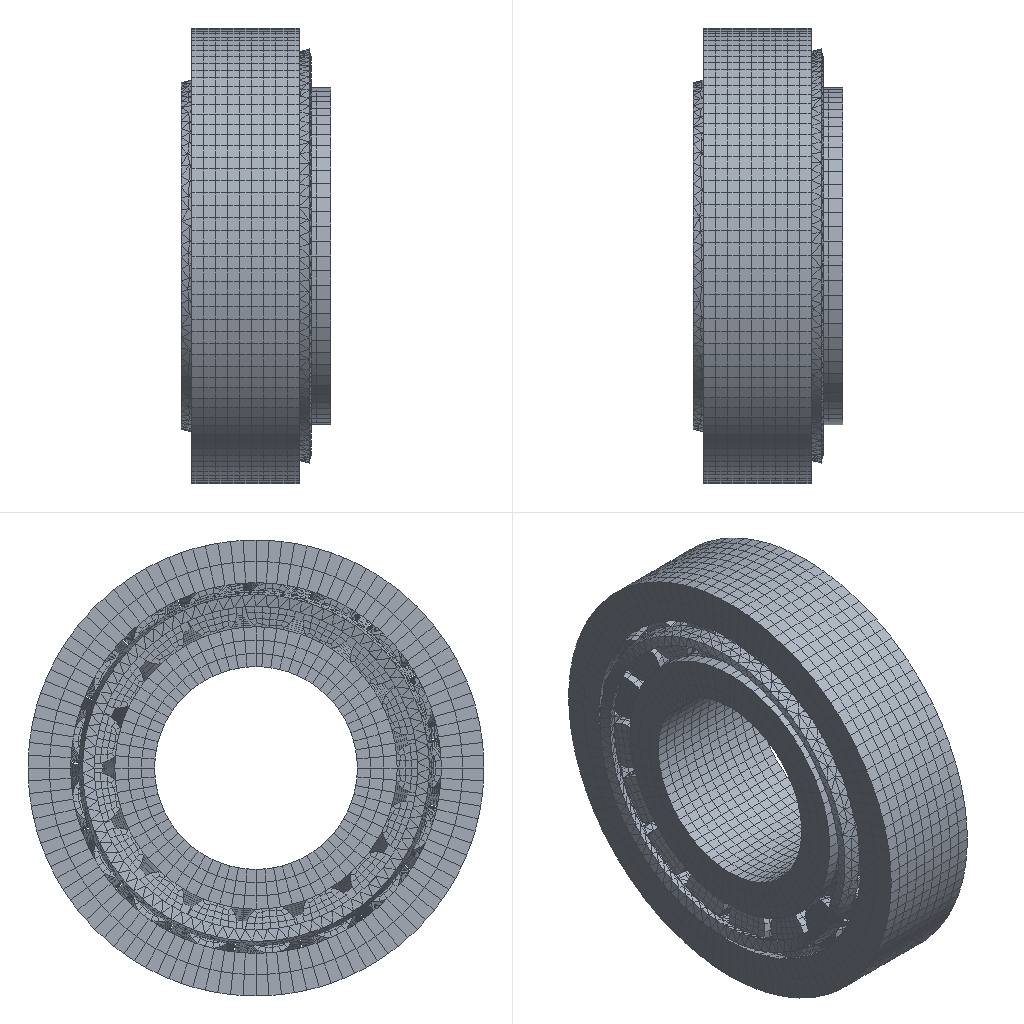Simulation study | abaqus
Set-up summary:
category,name,step,type,value,unit,region
solver,abaqus
solver,version,,,Abaqus/Explicit 2020
units,not stated in the deck,,not stated
analysis,deck,,transient,transient
load_step,Step-1,Step-1,transient
load_step,Step-2,Step-2,transient
load_step,Step-3,Step-3,transient
load_step,requested,,,3
mesh,nodes,,,23189
mesh,elements,,,18827
element_type,C3D4,,solid,3343
element_type,C3D8R,,solid,15484
load,load commands in deck,,count,4
bc,support commands in deck,,count,27
material,CAILIAO1,,in results
check,setup vs results,,match,"per instance, exact: element labels, types and connectivity; labels of the nodes the elements use; coordinates not compared"
Abaqus input file, long lists of numbers shortened:
*Heading
** Job name: Job-2 Model name: Model-1
** Generated by: Abaqus/CAE 2020
*Preprint, echo=NO, model=NO, history=NO, contact=NO
**
** PARTS
**
*Part, name=SKF_15578_15520_3
*Node
      1,   13.495,  -26.339,           0.
      2,   13.495,  -28.575,           0.
** (3358 more lines like these left out)
*Element, type=C3D8R
  1,  147, 1007, 2497,  575,    1,   20,  521,   75
  2, 1007,  156,  791, 2497,   20,    2,   21,  521
** (2014 more lines like these left out)
*Nset, nset=_PickedSet8, internal, generate
    1,  3360,     1
*Elset, elset=_PickedSet8, internal, generate
    1,  2016,     1
** Section: waiquan
*Solid Section, elset=_PickedSet8, material=cailiao1
,
*End Part
**
*Part, name=SKF_15578_15520_5
*Node
      1,   1.787,   17.127,           0.
      2,   1.169,   20.239,           0.
** (768 more lines like these left out)
*Element, type=C3D8R
  1, 165, 166, 498, 489,  13,  14, 124, 123
  2, 166,  18, 129, 498,  14,   1,  15, 124
** (570 more lines like these left out)
*Nset, nset=_PickedSet6, internal, generate
   1,  770,    1
*Elset, elset=_PickedSet6, internal, generate
   1,  572,    1
** Section: gongdongti
*Solid Section, elset=_PickedSet6, material=cailiao1
,
*End Part
**
*Part, name=SKF_15578_15520_23
*Node
      1,  0.7326,  -1.611,  -21.171
      2,  0.6985,           0.,  -21.223
** (1697 more lines like these left out)
*Element, type=C3D4
   1, 1652, 1601, 1637,  503
   2, 1652, 1404, 1405, 1601
** (3341 more lines like these left out)
*Nset, nset=_PickedSet6, internal, generate
    1,  1699,     1
*Elset, elset=_PickedSet6, internal, generate
    1,  3343,     1
** Section: baochijia
*Solid Section, elset=_PickedSet6, material=cailiao1
,
*End Part
**
*Part, name=SKF_15578_15520_25
*Node
      1,   13.796,   21.15,           0.
      2,   14.245,   19.205,           0.
** (5038 more lines like these left out)
*Element, type=C3D8R
  1,    2,  683,   62,    1,  163, 2595,  753,   63
  2,   57,   58,  702,  715,  770,  771, 2614, 2627
** (3742 more lines like these left out)
*Nset, nset=_PickedSet9, internal, generate
    1,  5040,     1
*Elset, elset=_PickedSet9, internal, generate
    1,  3744,     1
** Section: niequan
*Solid Section, elset=_PickedSet9, material=cailiao1
,
*End Part
**
**
** ASSEMBLY
**
*Assembly, name=Assembly
**
*Instance, name=SKF_15578_15520_25, part=SKF_15578_15520_25
          0.,           0.,           0.
          0.,           0.,           0.,           1.,           0.,           0.,         180.
*End Instance
**
*Instance, name=SKF_15578_15520_23, part=SKF_15578_15520_23
          0.,           0.,           0.
          0.,           0.,           0.,           1.,           0.,           0.,         180.
*End Instance
**
*Instance, name=SKF_15578_15520_5, part=SKF_15578_15520_5
          0.,           0.,           0.
          0.,           0.,           0.,           1.,           0.,           0.,         180.
*End Instance
**
*Instance, name=SKF_15578_15520_5_1, part=SKF_15578_15520_5
          0.,           0.,           0.
          0.,           0.,           0., 1.,           0.,           0., 201.176
*End Instance
**
*Instance, name=SKF_15578_15520_5_2, part=SKF_15578_15520_5
          0.,           0.,           0.
          0.,           0.,           0., 1.,           0.,           0., 222.353
*End Instance
**
*Instance, name=SKF_15578_15520_5_3, part=SKF_15578_15520_5
          0.,           0.,           0.
          0.,           0.,           0., -1.,           0.,           0., 116.471
*End Instance
**
*Instance, name=SKF_15578_15520_5_4, part=SKF_15578_15520_5
          0.,           0.,           0.
          0.,           0.,           0., -1.,           0.,           0., 95.294
*End Instance
**
*Instance, name=SKF_15578_15520_5_5, part=SKF_15578_15520_5
          0.,           0.,           0.
          0.,           0.,           0., -1.,           0.,           0., 74.118
*End Instance
**
*Instance, name=SKF_15578_15520_5_6, part=SKF_15578_15520_5
          0.,           0.,           0.
          0.,           0.,           0., -1.,           0.,           0., 52.941
*End Instance
**
*Instance, name=SKF_15578_15520_5_7, part=SKF_15578_15520_5
          0.,           0.,           0.
          0.,           0.,           0., -1.,           0.,           0., 31.765
*End Instance
**
*Instance, name=SKF_15578_15520_5_8, part=SKF_15578_15520_5
          0.,           0.,           0.
          0.,           0.,           0., -1.,           0.,           0., 10.588
*End Instance
**
*Instance, name=SKF_15578_15520_5_9, part=SKF_15578_15520_5
          0.,           0.,           0.
          0.,           0.,           0., 1.,           0.,           0., 10.588
*End Instance
**
*Instance, name=SKF_15578_15520_5_10, part=SKF_15578_15520_5
          0.,           0.,           0.
          0.,           0.,           0., 1.,           0.,           0., 31.765
*End Instance
**
*Instance, name=SKF_15578_15520_5_11, part=SKF_15578_15520_5
          0.,           0.,           0.
          0.,           0.,           0., 1.,           0.,           0., 52.941
*End Instance
**
*Instance, name=SKF_15578_15520_5_12, part=SKF_15578_15520_5
          0.,           0.,           0.
          0.,           0.,           0., 1.,           0.,           0., 74.118
*End Instance
**
*Instance, name=SKF_15578_15520_5_13, part=SKF_15578_15520_5
          0.,           0.,           0.
          0.,           0.,           0., 1.,           0.,           0., 95.294
*End Instance
**
*Instance, name=SKF_15578_15520_5_14, part=SKF_15578_15520_5
          0.,           0.,           0.
          0.,           0.,           0., 1.,           0.,           0., 116.471
*End Instance
**
*Instance, name=SKF_15578_15520_5_15, part=SKF_15578_15520_5
          0.,           0.,           0.
          0.,           0.,           0., 1.,           0.,           0., 137.647
*End Instance
**
*Instance, name=SKF_15578_15520_5_16, part=SKF_15578_15520_5
          0.,           0.,           0.
          0.,           0.,           0., 1.,           0.,           0., 158.824
*End Instance
**
*Instance, name=SKF_15578_15520_3, part=SKF_15578_15520_3
          0.,           0.,           0.
          0.,           0.,           0.,           1.,           0.,           0.,         180.
*End Instance
**
*Node
      1,   17.462, -4.4408921e-15,           0.
*Node
      2,   14.245, 2.9840975e-15,           0.
*Node
      3,           0.,           0.,          40.
*Node
      4,           0.,           0.,           0.
*Node
      5,   7.122, 1.49204875e-15,           0.
*Nset, nset=Set-7, instance=SKF_15578_15520_23
    6,    7,  110,  111,  152,  153,  154,  169,  170,  171,  172,  173,  174,  175,  176,  177
  178,  179,  180,  181,  182,  183,  184,  185,  186,  187,  188,  189,  190,  191,  192,  193
** (23 more lines like these left out)
*Elset, elset=Set-7, instance=SKF_15578_15520_23
    3,   46,   72,   81,   99,  106,  125,  222,  230,  238,  253,  273,  282,  289,  291,  293
  296,  297,  298,  301,  302,  304,  308,  319,  320,  325,  328,  329,  339,  341,  342,  348
** (23 more lines like these left out)
*Nset, nset=Set-8
 4,
*Nset, nset=Set-9
 2,
*Nset, nset=Set-10
 5,
*Nset, nset=m_Set-1
 1,
*Nset, nset=m_Set-8
 4,
*Nset, nset=m_Set-9
 2,
*Nset, nset=m_Set-10
 5,
*Nset, nset=ouhe-holder, instance=SKF_15578_15520_23, generate
    1,  1699,     1
*Elset, elset=ouhe-holder, instance=SKF_15578_15520_23, generate
    1,  3343,     1
*Nset, nset=_PickedSet53, internal
 2,
*Elset, elset=_Surf-1_S4, internal, instance=SKF_15578_15520_5_5
  49,  50,  51,  52,  53,  54,  55,  56,  57,  58,  59,  60,  61,  62,  63,  64
  65,  66,  73,  80, 192, 193, 194, 195, 196, 197, 198, 199, 200, 201, 202, 203
** (7 more lines like these left out)
*Elset, elset=_Surf-1_S3, internal, instance=SKF_15578_15520_5_5
   1,   2,   3,   4,   5,   6,   7,   8,   9,  10,  11,  12,  67,  68,  69,  70
  71,  72,  73,  74,  75,  76,  77,  78,  79,  80,  81,  82,  83, 102, 103, 104
** (9 more lines like these left out)
*Elset, elset=_Surf-1_S2, internal, instance=SKF_15578_15520_5_5
   1,   2,  13,  14,  15,  16,  17,  18,  49,  50,  51, 123, 124, 125, 144, 145
 156, 157, 158, 159, 160, 161, 192, 193, 194, 287, 288, 299, 300, 301, 302, 303
** (1 more lines like these left out)
*Surface, type=ELEMENT, name=Surf-1
_Surf-1_S4, S4
_Surf-1_S3, S3
_Surf-1_S2, S2
*Elset, elset=_Surf-2_S4, internal, instance=SKF_15578_15520_5_6
  49,  50,  51,  52,  53,  54,  55,  56,  57,  58,  59,  60,  61,  62,  63,  64
  65,  66,  73,  80, 192, 193, 194, 195, 196, 197, 198, 199, 200, 201, 202, 203
** (7 more lines like these left out)
*Elset, elset=_Surf-2_S3, internal, instance=SKF_15578_15520_5_6
   1,   2,   3,   4,   5,   6,   7,   8,   9,  10,  11,  12,  67,  68,  69,  70
  71,  72,  73,  74,  75,  76,  77,  78,  79,  80,  81,  82,  83, 102, 103, 104
** (9 more lines like these left out)
*Elset, elset=_Surf-2_S2, internal, instance=SKF_15578_15520_5_6
   1,   2,  13,  14,  15,  16,  17,  18,  49,  50,  51, 123, 124, 125, 144, 145
 156, 157, 158, 159, 160, 161, 192, 193, 194, 287, 288, 299, 300, 301, 302, 303
** (1 more lines like these left out)
*Surface, type=ELEMENT, name=Surf-2
_Surf-2_S4, S4
_Surf-2_S3, S3
_Surf-2_S2, S2
*Elset, elset=_Surf-3_S4, internal, instance=SKF_15578_15520_5_7
  49,  50,  51,  52,  53,  54,  55,  56,  57,  58,  59,  60,  61,  62,  63,  64
  65,  66,  73,  80, 192, 193, 194, 195, 196, 197, 198, 199, 200, 201, 202, 203
** (7 more lines like these left out)
*Elset, elset=_Surf-3_S3, internal, instance=SKF_15578_15520_5_7
   1,   2,   3,   4,   5,   6,   7,   8,   9,  10,  11,  12,  67,  68,  69,  70
  71,  72,  73,  74,  75,  76,  77,  78,  79,  80,  81,  82,  83, 102, 103, 104
** (9 more lines like these left out)
*Elset, elset=_Surf-3_S2, internal, instance=SKF_15578_15520_5_7
   1,   2,  13,  14,  15,  16,  17,  18,  49,  50,  51, 123, 124, 125, 144, 145
 156, 157, 158, 159, 160, 161, 192, 193, 194, 287, 288, 299, 300, 301, 302, 303
** (1 more lines like these left out)
*Surface, type=ELEMENT, name=Surf-3
_Surf-3_S4, S4
_Surf-3_S3, S3
_Surf-3_S2, S2
*Elset, elset=_Surf-4_S4, internal, instance=SKF_15578_15520_5_8
  49,  50,  51,  52,  53,  54,  55,  56,  57,  58,  59,  60,  61,  62,  63,  64
  65,  66,  73,  80, 192, 193, 194, 195, 196, 197, 198, 199, 200, 201, 202, 203
** (7 more lines like these left out)
*Elset, elset=_Surf-4_S3, internal, instance=SKF_15578_15520_5_8
   1,   2,   3,   4,   5,   6,   7,   8,   9,  10,  11,  12,  67,  68,  69,  70
  71,  72,  73,  74,  75,  76,  77,  78,  79,  80,  81,  82,  83, 102, 103, 104
** (9 more lines like these left out)
*Elset, elset=_Surf-4_S2, internal, instance=SKF_15578_15520_5_8
   1,   2,  13,  14,  15,  16,  17,  18,  49,  50,  51, 123, 124, 125, 144, 145
 156, 157, 158, 159, 160, 161, 192, 193, 194, 287, 288, 299, 300, 301, 302, 303
** (1 more lines like these left out)
*Surface, type=ELEMENT, name=Surf-4
_Surf-4_S4, S4
_Surf-4_S3, S3
_Surf-4_S2, S2
*Elset, elset=_Surf-5_S4, internal, instance=SKF_15578_15520_5_9
  49,  50,  51,  52,  53,  54,  55,  56,  57,  58,  59,  60,  61,  62,  63,  64
  65,  66,  73,  80, 192, 193, 194, 195, 196, 197, 198, 199, 200, 201, 202, 203
** (7 more lines like these left out)
*Elset, elset=_Surf-5_S3, internal, instance=SKF_15578_15520_5_9
   1,   2,   3,   4,   5,   6,   7,   8,   9,  10,  11,  12,  67,  68,  69,  70
  71,  72,  73,  74,  75,  76,  77,  78,  79,  80,  81,  82,  83, 102, 103, 104
** (9 more lines like these left out)
*Elset, elset=_Surf-5_S2, internal, instance=SKF_15578_15520_5_9
   1,   2,  13,  14,  15,  16,  17,  18,  49,  50,  51, 123, 124, 125, 144, 145
 156, 157, 158, 159, 160, 161, 192, 193, 194, 287, 288, 299, 300, 301, 302, 303
** (1 more lines like these left out)
*Surface, type=ELEMENT, name=Surf-5
_Surf-5_S4, S4
_Surf-5_S3, S3
_Surf-5_S2, S2
*Elset, elset=_Surf-6_S4, internal, instance=SKF_15578_15520_5_10
  49,  50,  51,  52,  53,  54,  55,  56,  57,  58,  59,  60,  61,  62,  63,  64
  65,  66,  73,  80, 192, 193, 194, 195, 196, 197, 198, 199, 200, 201, 202, 203
** (7 more lines like these left out)
*Elset, elset=_Surf-6_S3, internal, instance=SKF_15578_15520_5_10
   1,   2,   3,   4,   5,   6,   7,   8,   9,  10,  11,  12,  67,  68,  69,  70
  71,  72,  73,  74,  75,  76,  77,  78,  79,  80,  81,  82,  83, 102, 103, 104
** (9 more lines like these left out)
*Elset, elset=_Surf-6_S2, internal, instance=SKF_15578_15520_5_10
   1,   2,  13,  14,  15,  16,  17,  18,  49,  50,  51, 123, 124, 125, 144, 145
 156, 157, 158, 159, 160, 161, 192, 193, 194, 287, 288, 299, 300, 301, 302, 303
** (1 more lines like these left out)
*Surface, type=ELEMENT, name=Surf-6
_Surf-6_S4, S4
_Surf-6_S3, S3
_Surf-6_S2, S2
*Elset, elset=_Surf-7_S4, internal, instance=SKF_15578_15520_5_11
  49,  50,  51,  52,  53,  54,  55,  56,  57,  58,  59,  60,  61,  62,  63,  64
  65,  66,  73,  80, 192, 193, 194, 195, 196, 197, 198, 199, 200, 201, 202, 203
** (7 more lines like these left out)
*Elset, elset=_Surf-7_S3, internal, instance=SKF_15578_15520_5_11
   1,   2,   3,   4,   5,   6,   7,   8,   9,  10,  11,  12,  67,  68,  69,  70
  71,  72,  73,  74,  75,  76,  77,  78,  79,  80,  81,  82,  83, 102, 103, 104
** (9 more lines like these left out)
*Elset, elset=_Surf-7_S2, internal, instance=SKF_15578_15520_5_11
   1,   2,  13,  14,  15,  16,  17,  18,  49,  50,  51, 123, 124, 125, 144, 145
 156, 157, 158, 159, 160, 161, 192, 193, 194, 287, 288, 299, 300, 301, 302, 303
** (1 more lines like these left out)
*Surface, type=ELEMENT, name=Surf-7
_Surf-7_S4, S4
_Surf-7_S3, S3
_Surf-7_S2, S2
*Elset, elset=_Surf-8_S4, internal, instance=SKF_15578_15520_5_12
  49,  50,  51,  52,  53,  54,  55,  56,  57,  58,  59,  60,  61,  62,  63,  64
  65,  66,  73,  80, 192, 193, 194, 195, 196, 197, 198, 199, 200, 201, 202, 203
** (7 more lines like these left out)
*Elset, elset=_Surf-8_S3, internal, instance=SKF_15578_15520_5_12
   1,   2,   3,   4,   5,   6,   7,   8,   9,  10,  11,  12,  67,  68,  69,  70
  71,  72,  73,  74,  75,  76,  77,  78,  79,  80,  81,  82,  83, 102, 103, 104
** (9 more lines like these left out)
*Elset, elset=_Surf-8_S2, internal, instance=SKF_15578_15520_5_12
   1,   2,  13,  14,  15,  16,  17,  18,  49,  50,  51, 123, 124, 125, 144, 145
 156, 157, 158, 159, 160, 161, 192, 193, 194, 287, 288, 299, 300, 301, 302, 303
** (1 more lines like these left out)
*Surface, type=ELEMENT, name=Surf-8
_Surf-8_S4, S4
_Surf-8_S3, S3
_Surf-8_S2, S2
*Elset, elset=_Surf-9_S4, internal, instance=SKF_15578_15520_5_13
  49,  50,  51,  52,  53,  54,  55,  56,  57,  58,  59,  60,  61,  62,  63,  64
  65,  66,  73,  80, 192, 193, 194, 195, 196, 197, 198, 199, 200, 201, 202, 203
** (7 more lines like these left out)
*Elset, elset=_Surf-9_S3, internal, instance=SKF_15578_15520_5_13
   1,   2,   3,   4,   5,   6,   7,   8,   9,  10,  11,  12,  67,  68,  69,  70
  71,  72,  73,  74,  75,  76,  77,  78,  79,  80,  81,  82,  83, 102, 103, 104
** (9 more lines like these left out)
*Elset, elset=_Surf-9_S2, internal, instance=SKF_15578_15520_5_13
   1,   2,  13,  14,  15,  16,  17,  18,  49,  50,  51, 123, 124, 125, 144, 145
 156, 157, 158, 159, 160, 161, 192, 193, 194, 287, 288, 299, 300, 301, 302, 303
** (1 more lines like these left out)
*Surface, type=ELEMENT, name=Surf-9
_Surf-9_S4, S4
_Surf-9_S3, S3
_Surf-9_S2, S2
*Elset, elset=_Surf-10_S4, internal, instance=SKF_15578_15520_5_14
  49,  50,  51,  52,  53,  54,  55,  56,  57,  58,  59,  60,  61,  62,  63,  64
  65,  66,  73,  80, 192, 193, 194, 195, 196, 197, 198, 199, 200, 201, 202, 203
** (7 more lines like these left out)
*Elset, elset=_Surf-10_S3, internal, instance=SKF_15578_15520_5_14
   1,   2,   3,   4,   5,   6,   7,   8,   9,  10,  11,  12,  67,  68,  69,  70
  71,  72,  73,  74,  75,  76,  77,  78,  79,  80,  81,  82,  83, 102, 103, 104
** (9 more lines like these left out)
*Elset, elset=_Surf-10_S2, internal, instance=SKF_15578_15520_5_14
   1,   2,  13,  14,  15,  16,  17,  18,  49,  50,  51, 123, 124, 125, 144, 145
 156, 157, 158, 159, 160, 161, 192, 193, 194, 287, 288, 299, 300, 301, 302, 303
** (1 more lines like these left out)
*Surface, type=ELEMENT, name=Surf-10
_Surf-10_S4, S4
_Surf-10_S3, S3
_Surf-10_S2, S2
*Elset, elset=_Surf-11_S4, internal, instance=SKF_15578_15520_5_15
  49,  50,  51,  52,  53,  54,  55,  56,  57,  58,  59,  60,  61,  62,  63,  64
  65,  66,  73,  80, 192, 193, 194, 195, 196, 197, 198, 199, 200, 201, 202, 203
** (7 more lines like these left out)
*Elset, elset=_Surf-11_S3, internal, instance=SKF_15578_15520_5_15
   1,   2,   3,   4,   5,   6,   7,   8,   9,  10,  11,  12,  67,  68,  69,  70
  71,  72,  73,  74,  75,  76,  77,  78,  79,  80,  81,  82,  83, 102, 103, 104
** (9 more lines like these left out)
*Elset, elset=_Surf-11_S2, internal, instance=SKF_15578_15520_5_15
   1,   2,  13,  14,  15,  16,  17,  18,  49,  50,  51, 123, 124, 125, 144, 145
 156, 157, 158, 159, 160, 161, 192, 193, 194, 287, 288, 299, 300, 301, 302, 303
** (1 more lines like these left out)
*Surface, type=ELEMENT, name=Surf-11
_Surf-11_S4, S4
_Surf-11_S3, S3
_Surf-11_S2, S2
*Elset, elset=_Surf-12_S4, internal, instance=SKF_15578_15520_5_16
  49,  50,  51,  52,  53,  54,  55,  56,  57,  58,  59,  60,  61,  62,  63,  64
  65,  66,  73,  80, 192, 193, 194, 195, 196, 197, 198, 199, 200, 201, 202, 203
** (7 more lines like these left out)
*Elset, elset=_Surf-12_S3, internal, instance=SKF_15578_15520_5_16
   1,   2,   3,   4,   5,   6,   7,   8,   9,  10,  11,  12,  67,  68,  69,  70
  71,  72,  73,  74,  75,  76,  77,  78,  79,  80,  81,  82,  83, 102, 103, 104
** (9 more lines like these left out)
*Elset, elset=_Surf-12_S2, internal, instance=SKF_15578_15520_5_16
   1,   2,  13,  14,  15,  16,  17,  18,  49,  50,  51, 123, 124, 125, 144, 145
 156, 157, 158, 159, 160, 161, 192, 193, 194, 287, 288, 299, 300, 301, 302, 303
** (1 more lines like these left out)
*Surface, type=ELEMENT, name=Surf-12
_Surf-12_S4, S4
_Surf-12_S3, S3
_Surf-12_S2, S2
*Elset, elset=_Surf-13_S4, internal, instance=SKF_15578_15520_5
  49,  50,  51,  52,  53,  54,  55,  56,  57,  58,  59,  60,  61,  62,  63,  64
  65,  66,  73,  80, 192, 193, 194, 195, 196, 197, 198, 199, 200, 201, 202, 203
** (7 more lines like these left out)
*Elset, elset=_Surf-13_S3, internal, instance=SKF_15578_15520_5
   1,   2,   3,   4,   5,   6,   7,   8,   9,  10,  11,  12,  67,  68,  69,  70
  71,  72,  73,  74,  75,  76,  77,  78,  79,  80,  81,  82,  83, 102, 103, 104
** (9 more lines like these left out)
*Elset, elset=_Surf-13_S2, internal, instance=SKF_15578_15520_5
   1,   2,  13,  14,  15,  16,  17,  18,  49,  50,  51, 123, 124, 125, 144, 145
 156, 157, 158, 159, 160, 161, 192, 193, 194, 287, 288, 299, 300, 301, 302, 303
** (1 more lines like these left out)
*Surface, type=ELEMENT, name=Surf-13
_Surf-13_S4, S4
_Surf-13_S3, S3
_Surf-13_S2, S2
*Elset, elset=_Surf-14_S4, internal, instance=SKF_15578_15520_5_1
  49,  50,  51,  52,  53,  54,  55,  56,  57,  58,  59,  60,  61,  62,  63,  64
  65,  66,  73,  80, 192, 193, 194, 195, 196, 197, 198, 199, 200, 201, 202, 203
** (7 more lines like these left out)
*Elset, elset=_Surf-14_S3, internal, instance=SKF_15578_15520_5_1
   1,   2,   3,   4,   5,   6,   7,   8,   9,  10,  11,  12,  67,  68,  69,  70
  71,  72,  73,  74,  75,  76,  77,  78,  79,  80,  81,  82,  83, 102, 103, 104
** (9 more lines like these left out)
*Elset, elset=_Surf-14_S2, internal, instance=SKF_15578_15520_5_1
   1,   2,  13,  14,  15,  16,  17,  18,  49,  50,  51, 123, 124, 125, 144, 145
 156, 157, 158, 159, 160, 161, 192, 193, 194, 287, 288, 299, 300, 301, 302, 303
** (1 more lines like these left out)
*Surface, type=ELEMENT, name=Surf-14
_Surf-14_S4, S4
_Surf-14_S3, S3
_Surf-14_S2, S2
*Elset, elset=_Surf-15_S4, internal, instance=SKF_15578_15520_5_2
  49,  50,  51,  52,  53,  54,  55,  56,  57,  58,  59,  60,  61,  62,  63,  64
  65,  66,  73,  80, 192, 193, 194, 195, 196, 197, 198, 199, 200, 201, 202, 203
** (7 more lines like these left out)
*Elset, elset=_Surf-15_S3, internal, instance=SKF_15578_15520_5_2
   1,   2,   3,   4,   5,   6,   7,   8,   9,  10,  11,  12,  67,  68,  69,  70
  71,  72,  73,  74,  75,  76,  77,  78,  79,  80,  81,  82,  83, 102, 103, 104
** (9 more lines like these left out)
*Elset, elset=_Surf-15_S2, internal, instance=SKF_15578_15520_5_2
   1,   2,  13,  14,  15,  16,  17,  18,  49,  50,  51, 123, 124, 125, 144, 145
 156, 157, 158, 159, 160, 161, 192, 193, 194, 287, 288, 299, 300, 301, 302, 303
** (1 more lines like these left out)
*Surface, type=ELEMENT, name=Surf-15
_Surf-15_S4, S4
_Surf-15_S3, S3
_Surf-15_S2, S2
*Elset, elset=_Surf-16_S4, internal, instance=SKF_15578_15520_5_3
  49,  50,  51,  52,  53,  54,  55,  56,  57,  58,  59,  60,  61,  62,  63,  64
  65,  66,  73,  80, 192, 193, 194, 195, 196, 197, 198, 199, 200, 201, 202, 203
** (7 more lines like these left out)
*Elset, elset=_Surf-16_S3, internal, instance=SKF_15578_15520_5_3
   1,   2,   3,   4,   5,   6,   7,   8,   9,  10,  11,  12,  67,  68,  69,  70
  71,  72,  73,  74,  75,  76,  77,  78,  79,  80,  81,  82,  83, 102, 103, 104
** (9 more lines like these left out)
*Elset, elset=_Surf-16_S2, internal, instance=SKF_15578_15520_5_3
   1,   2,  13,  14,  15,  16,  17,  18,  49,  50,  51, 123, 124, 125, 144, 145
 156, 157, 158, 159, 160, 161, 192, 193, 194, 287, 288, 299, 300, 301, 302, 303
** (1 more lines like these left out)
*Surface, type=ELEMENT, name=Surf-16
_Surf-16_S4, S4
_Surf-16_S3, S3
_Surf-16_S2, S2
*Elset, elset=_Surf-17_S4, internal, instance=SKF_15578_15520_5_4
  49,  50,  51,  52,  53,  54,  55,  56,  57,  58,  59,  60,  61,  62,  63,  64
  65,  66,  73,  80, 192, 193, 194, 195, 196, 197, 198, 199, 200, 201, 202, 203
** (7 more lines like these left out)
*Elset, elset=_Surf-17_S3, internal, instance=SKF_15578_15520_5_4
   1,   2,   3,   4,   5,   6,   7,   8,   9,  10,  11,  12,  67,  68,  69,  70
  71,  72,  73,  74,  75,  76,  77,  78,  79,  80,  81,  82,  83, 102, 103, 104
** (9 more lines like these left out)
*Elset, elset=_Surf-17_S2, internal, instance=SKF_15578_15520_5_4
   1,   2,  13,  14,  15,  16,  17,  18,  49,  50,  51, 123, 124, 125, 144, 145
 156, 157, 158, 159, 160, 161, 192, 193, 194, 287, 288, 299, 300, 301, 302, 303
** (1 more lines like these left out)
*Surface, type=ELEMENT, name=Surf-17
_Surf-17_S4, S4
_Surf-17_S3, S3
_Surf-17_S2, S2
*Elset, elset=_Surf-niequan_S5, internal, instance=SKF_15578_15520_25
    7,   18,   28,   32,   33,   35,   37,   59,   70,   80,   84,   85,   87,   89,  111,  122
  132,  136,  137,  139,  141,  163,  174,  184,  188,  189,  191,  193,  215,  226,  236,  240
** (30 more lines like these left out)
*Elset, elset=_Surf-niequan_S6, internal, instance=SKF_15578_15520_25, generate
   45,  3737,    52
*Surface, type=ELEMENT, name=Surf-niequan
_Surf-niequan_S5, S5
_Surf-niequan_S6, S6
*Elset, elset=_Surf-waiquan_S6, internal, instance=SKF_15578_15520_3
    1,    3,    5,    7,    9,   11,   13,   15,   17,   19,   21,   23,   25,   27,   29,   31
   33,   35,   37,   39,   41,   43,   45,   47,   49,   51,   53,   55,   57,   59,   61,   63
** (30 more lines like these left out)
*Elset, elset=_Surf-waiquan_S4, internal, instance=SKF_15578_15520_3
  506,  508,  510,  512,  514,  516,  518,  520,  522,  524,  526,  528,  530,  532,  534,  536
  538,  540,  542,  544,  546,  548,  550,  552,  554,  556,  558,  560,  562,  564,  566,  568
** (30 more lines like these left out)
*Surface, type=ELEMENT, name=Surf-waiquan
_Surf-waiquan_S6, S6
_Surf-waiquan_S4, S4
*Elset, elset=_s_Surf-23_S3, internal, instance=SKF_15578_15520_23
    2,   15,   22,   26,   32,   37,   49,   56,   69,   74,   86,   96,   98,  100,  107,  111
  114,  127,  131,  140,  149,  162,  164,  165,  167,  173,  186,  191,  197,  202,  205,  207
** (5 more lines like these left out)
*Elset, elset=_s_Surf-23_S1, internal, instance=SKF_15578_15520_23
   19,  222,  255,  257,  286,  307,  400,  404,  409,  411,  412,  423,  430,  440,  442,  445
  448,  458,  462,  473,  476,  486,  490,  499,  526,  533,  538,  553,  554,  582,  600,  604
** (18 more lines like these left out)
*Elset, elset=_s_Surf-23_S4, internal, instance=SKF_15578_15520_23
  137,  144,  153,  258,  303,  405,  414,  421,  429,  432,  435,  439,  443,  444,  446,  449
  454,  461,  477,  481,  500,  503,  504,  507,  513,  516,  522,  525,  530,  535,  549,  551
** (9 more lines like these left out)
*Elset, elset=_s_Surf-23_S2, internal, instance=SKF_15578_15520_23
  313,  396,  397,  416,  418,  424,  431,  433,  434,  455,  456,  457,  459,  469,  470,  480
  498,  512,  524,  528,  532,  542,  546,  548,  562,  564,  566,  574,  578,  583,  588,  594
** (20 more lines like these left out)
*Surface, type=ELEMENT, name=s_Surf-23
_s_Surf-23_S3, S3
_s_Surf-23_S1, S1
_s_Surf-23_S4, S4
_s_Surf-23_S2, S2
*Elset, elset=__PickedSurf44_S4, internal, instance=SKF_15578_15520_25
    6,    9,   14,   20,   36,   58,   61,   66,   72,   88,  110,  113,  118,  124,  140,  162
  165,  170,  176,  192,  214,  217,  222,  228,  244,  266,  269,  274,  280,  296,  318,  321
** (21 more lines like these left out)
*Elset, elset=__PickedSurf44_S6, internal, instance=SKF_15578_15520_25
   12,   15,   16,   19,   21,   22,   23,   64,   67,   68,   71,   73,   74,   75,  116,  119
  120,  123,  125,  126,  127,  168,  171,  172,  175,  177,  178,  179,  220,  223,  224,  227
** (30 more lines like these left out)
*Surface, type=ELEMENT, name=_PickedSurf44, internal
__PickedSurf44_S4, S4
__PickedSurf44_S6, S6
*Elset, elset=__PickedSurf52_S3, internal, instance=SKF_15578_15520_23
    2,    4,    7,    8,    9,   14,   15,   19,   22,   25,   26,   32,   34,   37,   38,   45
   46,   49,   51,   55,   56,   61,   62,   64,   68,   69,   70,   71,   72,   74,   76,   79
** (91 more lines like these left out)
*Elset, elset=__PickedSurf52_S1, internal, instance=SKF_15578_15520_23
    3,   19,  193,  222,  231,  255,  257,  265,  286,  294,  301,  304,  305,  307,  312,  316
  319,  325,  326,  328,  329,  333,  335,  337,  338,  339,  340,  341,  342,  345,  347,  348
** (41 more lines like these left out)
*Elset, elset=__PickedSurf52_S4, internal, instance=SKF_15578_15520_23
  137,  144,  153,  222,  258,  263,  279,  281,  283,  284,  287,  292,  302,  303,  310,  320
  358,  363,  366,  369,  371,  380,  384,  393,  399,  401,  405,  407,  414,  421,  429,  432
** (34 more lines like these left out)
*Elset, elset=__PickedSurf52_S2, internal, instance=SKF_15578_15520_23
  106,  261,  265,  293,  298,  311,  313,  330,  362,  375,  389,  390,  394,  395,  396,  397
  398,  402,  406,  408,  416,  418,  424,  428,  431,  433,  434,  455,  456,  457,  459,  469
** (39 more lines like these left out)
*Surface, type=ELEMENT, name=_PickedSurf52, internal
__PickedSurf52_S3, S3
__PickedSurf52_S1, S1
__PickedSurf52_S4, S4
__PickedSurf52_S2, S2
*Elset, elset=__PickedSurf54_S6, internal, instance=SKF_15578_15520_3
  505,  507,  509,  511,  513,  515,  517,  519,  521,  523,  525,  527,  529,  531,  533,  535
  537,  539,  541,  543,  545,  547,  549,  551,  553,  555,  557,  559,  561,  563,  565,  567
** (30 more lines like these left out)
*Elset, elset=__PickedSurf54_S4, internal, instance=SKF_15578_15520_3
    2,    4,    6,    8,   10,   12,   14,   16,   18,   20,   22,   24,   26,   28,   30,   32
   34,   36,   38,   40,   42,   44,   46,   48,   50,   52,   54,   56,   58,   60,   62,   64
** (30 more lines like these left out)
*Surface, type=ELEMENT, name=_PickedSurf54, internal
__PickedSurf54_S6, S6
__PickedSurf54_S4, S4
** Constraint: Constraint-1
*Coupling, constraint name=Constraint-1, ref node=m_Set-9, surface=_PickedSurf44
*Kinematic
** Constraint: Constraint-3
*Coupling, constraint name=Constraint-3, ref node=m_Set-8, surface=_PickedSurf54
*Kinematic
** Constraint: Constraint-4
*Coupling, constraint name=Constraint-4, ref node=m_Set-10, surface=s_Surf-23
*Kinematic
*End Assembly
*Amplitude, name=Amp-1, definition=SMOOTH STEP
             0.,              0.,           0.005,              1.
*Amplitude, name=Amp-2, definition=SMOOTH STEP
             0.,              0.,           0.002,              1.
*Amplitude, name=Amp-3
             0.,              0.,            0.05,              1.
*Amplitude, name=Amp-4, time=TOTAL TIME, definition=SMOOTH STEP
             0.,              0.,           0.003,              1.
**
** MATERIALS
**
*Material, name=cailiao1
*Density
 7.85e-09,
*Elastic
206000., 0.3
**
** INTERACTION PROPERTIES
**
*Surface Interaction, name=IntProp-1
*Friction, exponential decay
0.1, 0.05, 0.01
*Surface Behavior, pressure-overclosure=HARD
*Surface Interaction, name=IntProp-2
*Friction
 0.002,
*Surface Behavior, pressure-overclosure=HARD
**
** BOUNDARY CONDITIONS
**
** Name: BC-4 Type: 位移/转角
*Boundary
Set-8, 1, 1
Set-8, 2, 2
Set-8, 3, 3
Set-8, 4, 4
Set-8, 5, 5
Set-8, 6, 6
**
** INTERACTIONS
**
** Interaction: Int-36
*Contact, op=NEW
*Contact Inclusions, ALL EXTERIOR
*Contact Property Assignment
 ,  , IntProp-2
** ----------------------------------------------------------------
**
** STEP: Step-1
**
*Step, name=Step-1, nlgeom=YES
*Dynamic, Explicit
, 0.001
*Bulk Viscosity
0.06, 1.2
**
** BOUNDARY CONDITIONS
**
** Name: [REDACTED] : Displacement/rotation angle
*Boundary
Set-10, 1, 1
Set-10, 4, 4
Set-10, 5, 5
Set-10, 6, 6
** Name: [REDACTED] : Speed/Angular velocity
*Boundary, type=VELOCITY
Set-9, 1, 1
Set-9, 4, 4
Set-9, 5, 5
Set-9, 6, 6
**
** LOADS
**
** Name: Load-G   Type: Gravity
*Dload
, GRAV, 9800., 0., 1., 0.
**
** OUTPUT REQUESTS
**
*Restart, write, number interval=1, time marks=NO
**
** FIELD OUTPUT: F-Output-1
**
*Output, field
*Node Output
CF, RF, RT, U, UR, V, VR
*Element Output, directions=YES
E, LE, MISES, NFORC, S, SF
*Contact Output
CDISP, CSTRESS
**
** HISTORY OUTPUT: H-Output-1
**
*Output, history
*Node Output, nset=Set-8
RF1, RF2, RF3, RM1, RM2, RM3
**
** HISTORY OUTPUT: H-Output-2
**
*Node Output, nset=Set-9
U1, U2, U3, UR1, UR2, UR3, V1, V2
V3, VR1, VR2, VR3
*End Step
** ----------------------------------------------------------------
**
** STEP: Step-2
**
*Step, name=Step-2, nlgeom=YES
*Dynamic, Explicit
, 0.001
*Bulk Viscosity
0.06, 1.2
**
** LOADS
**
** Name: Load-1   Type: Concentrated force
*Cload, amplitude=Amp-4
Set-9, 1, 0.
Set-9, 2, 50000.
**
** OUTPUT REQUESTS
**
*Restart, write, number interval=1, time marks=NO
**
** FIELD OUTPUT: F-Output-1
**
*Output, field
*Node Output
CF, RF, RT, U, UR, V, VR
*Element Output, directions=YES
E, LE, MISES, NFORC, S, SF
*Contact Output
CDISP, CSTRESS
**
** HISTORY OUTPUT: H-Output-1
**
*Output, history
*Node Output, nset=Set-8
RF1, RF2, RF3, RM1, RM2, RM3
**
** HISTORY OUTPUT: H-Output-2
**
*Node Output, nset=Set-9
U1, U2, U3, UR1, UR2, UR3, V1, V2
V3, VR1, VR2, VR3
*End Step
** ----------------------------------------------------------------
**
** STEP: Step-3
**
*Step, name=Step-3, nlgeom=YES
*Dynamic, Explicit
, 0.045
*Bulk Viscosity
0.06, 1.2
**
** BOUNDARY CONDITIONS
**
** Name: BC-4 Type: 位移/转角
*Boundary, op=NEW
Set-8, 1, 1
Set-8, 2, 2
Set-8, 3, 3
Set-8, 4, 4
Set-8, 5, 5
Set-8, 6, 6
** Name: [REDACTED] : Displacement/rotation angle
*Boundary, op=NEW
Set-10, 1, 1
Set-10, 5, 5
Set-10, 6, 6
** Name: [REDACTED] : Speed/Angular velocity
*Boundary, op=NEW, type=VELOCITY
Set-9, 1, 1
Set-9, 4, 4, 120.
Set-9, 5, 5
Set-9, 6, 6
**
** OUTPUT REQUESTS
**
*Restart, write, number interval=1, time marks=NO
**
** FIELD OUTPUT: F-Output-1
**
*Output, field, number interval=100
*Node Output
CF, RF, RT, U, UR, V, VR
*Element Output, directions=YES
E, LE, MISES, NFORC, S, SF
*Contact Output
CDISP, CSTRESS
**
** HISTORY OUTPUT: H-Output-1
**
*Output, history, time interval=2.25e-05
*Node Output, nset=Set-8
RF1, RF2, RF3, RM1, RM2, RM3
**
** HISTORY OUTPUT: H-Output-2
**
*Node Output, nset=Set-9
U1, U2, U3, UR1, UR2, UR3, V1, V2
V3, VR1, VR2, VR3
*End Step
Results summary:
result,step,Step-1,completed,increments=15830 time=0.001/0.001
result,step,Step-2,completed,increments=15822 time=0.001/0.001
result,step,Step-3,partial,increments=647529 time=0.03488/0.045
result,analysis,,,transient
result,last_loadstep,,,3
result,primary field,,,U
result,reaction total,,FX,270.712,model units
result,reaction total,,FY,-49528.402,model units
result,reaction total,,FZ,180.895,model units